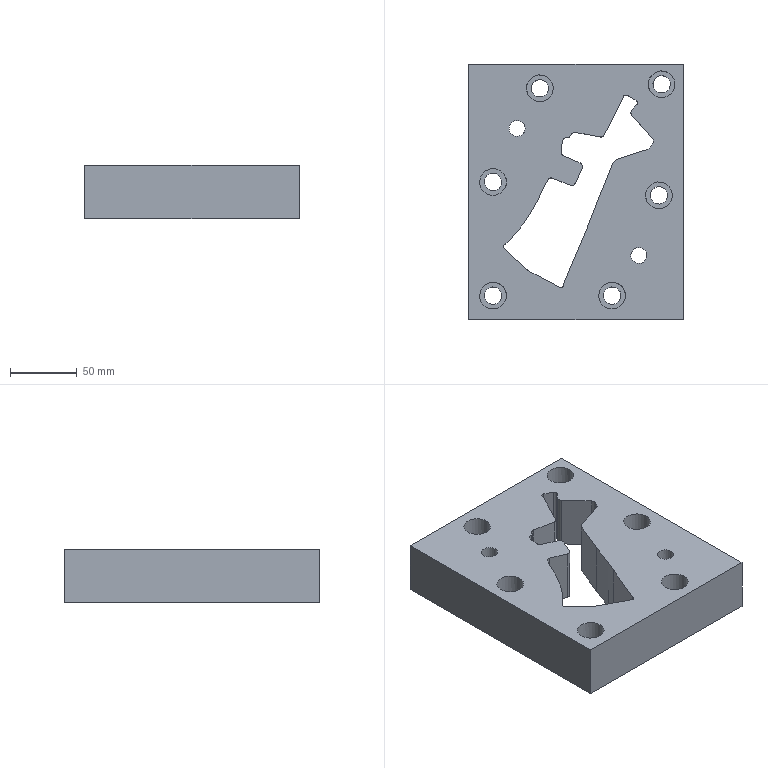Part | STEP file | gslz 2016.10.28-13_id110_x_t | 1 solid | 76 faces | box 160 x 191 x 40 mm | volume 949174 mm3 | plane 41 | cylinder 35 | commonest cylinder face diameters 4 x9 6 x6 13 x6 20 x6 8 x2 12 x2